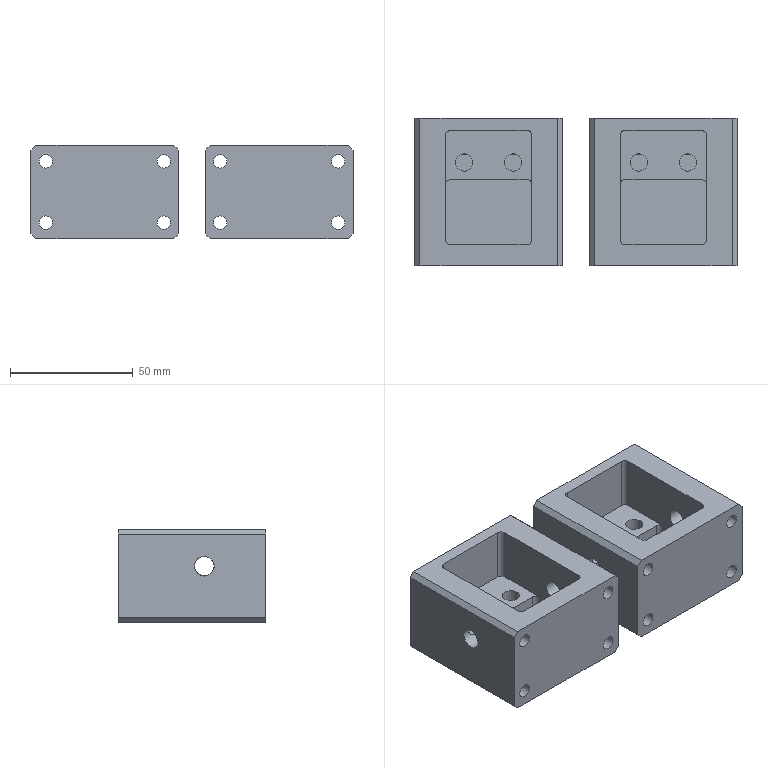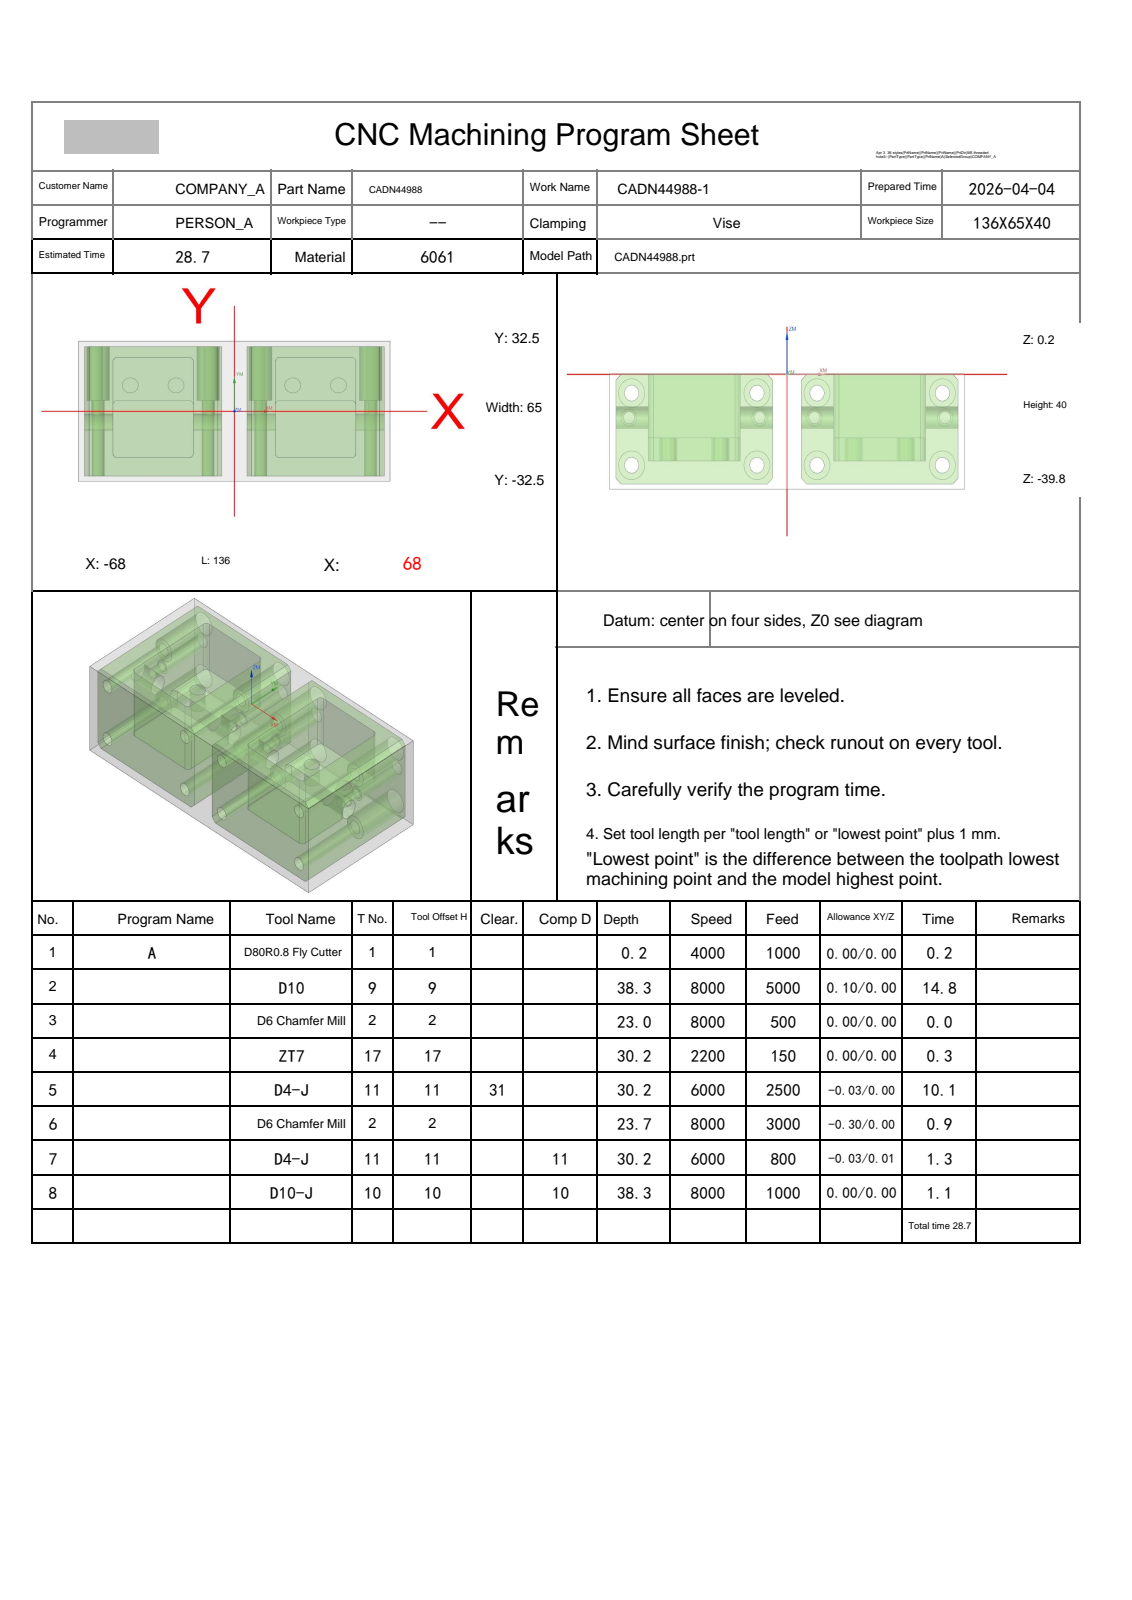NC program | NX | posted by the shop | part box 131 x 60 x 38 mm
Lines 4540 to 5571 of 30516:
N5 T11 M06
(D4-J  D=4. R=0. H=11 ce=0.00 di=0.01)
G00 G90 G54 X47.547 Y-18.9 M03 S6000
G43 H11 Z20.
M08
Z.303
G01 X47.548 Y-18.907 Z.217 F2000.
X47.551 Y-18.926 Z.139
X47.556 Y-18.955 Z.069
X47.564 Y-18.994 Z.007
X47.575 Y-19.039 Z-.049
X47.589 Y-19.09 Z-.098
X47.606 Y-19.144 Z-.141
X47.627 Y-19.2 Z-.177
X47.651 Y-19.256 Z-.208
X47.68 Y-19.31 Z-.234
X47.712 Y-19.361 Z-.255
X47.749 Y-19.406 Z-.271
X47.791 Y-19.445 Z-.283
X47.838 Y-19.474 Z-.291
X47.89 Y-19.493 Z-.296
X47.947 Y-19.5 Z-.297
X51.1 F2500.
Y-16.347
X51.084 Y-16.304 Z-.298
X51.038 Y-16.282 Z-.301
X50.966 Y-16.28 Z-.305
X50.871 Y-16.297 Z-.31
X50.756 Y-16.33 Z-.317
X50.626 Y-16.379 Z-.325
X50.482 Y-16.441 Z-.334
X50.33 Y-16.516 Z-.344
X50.171 Y-16.6 Z-.355
X50.01 Y-16.693 Z-.366
X49.85 Y-16.794 Z-.378
X49.512 Y-17.035 Z-.404
X49.197 Y-17.303 Z-.432
X48.905 Y-17.595 Z-.46
X48.638 Y-17.911 Z-.487
X48.397 Y-18.249 Z-.514
X48.296 Y-18.409 Z-.526
X48.202 Y-18.57 Z-.537
X48.117 Y-18.729 Z-.547
X48.043 Y-18.882 Z-.557
X47.98 Y-19.025 Z-.566
X47.931 Y-19.156 Z-.574
X47.898 Y-19.271 Z-.581
X47.881 Y-19.366 Z-.587
X47.882 Y-19.438 Z-.591
X47.904 Y-19.484 Z-.594
X47.947 Y-19.5
X51.1
Y-16.347
X51.084 Y-16.304 Z-.595
X51.038 Y-16.282 Z-.598
X50.966 Y-16.28 Z-.602
X50.871 Y-16.296 Z-.608
X50.756 Y-16.33 Z-.615
X50.626 Y-16.378 Z-.623
X50.482 Y-16.44 Z-.632
X50.329 Y-16.514 Z-.642
X50.171 Y-16.598 Z-.652
X50.01 Y-16.691 Z-.663
X49.85 Y-16.791 Z-.675
X49.512 Y-17.033 Z-.702
X49.197 Y-17.3 Z-.729
X48.905 Y-17.593 Z-.757
X48.638 Y-17.909 Z-.785
X48.397 Y-18.247 Z-.811
X48.296 Y-18.408 Z-.823
X48.202 Y-18.569 Z-.834
X48.117 Y-18.728 Z-.845
X48.043 Y-18.881 Z-.855
X47.98 Y-19.025 Z-.864
X47.931 Y-19.156 Z-.872
X47.898 Y-19.27 Z-.878
X47.881 Y-19.366 Z-.884
X47.882 Y-19.438 Z-.888
X47.904 Y-19.484 Z-.891
X47.947 Y-19.5 Z-.892
X51.1
Y-16.347
X51.084 Y-16.304 Z-.893
X51.038 Y-16.282 Z-.895
X50.966 Y-16.28 Z-.899
X50.871 Y-16.296 Z-.905
X50.756 Y-16.329 Z-.912
X50.625 Y-16.377 Z-.92
X50.482 Y-16.438 Z-.929
X50.329 Y-16.512 Z-.939
X50.171 Y-16.596 Z-.949
X50.01 Y-16.689 Z-.961
X49.85 Y-16.789 Z-.972
X49.512 Y-17.03 Z-.999
X49.197 Y-17.297 Z-1.026
X48.905 Y-17.59 Z-1.054
X48.638 Y-17.907 Z-1.082
X48.396 Y-18.246 Z-1.108
X48.296 Y-18.406 Z-1.12
X48.202 Y-18.568 Z-1.131
X48.117 Y-18.727 Z-1.142
X48.043 Y-18.88 Z-1.152
X47.98 Y-19.024 Z-1.161
X47.931 Y-19.155 Z-1.169
X47.898 Y-19.27 Z-1.176
X47.881 Y-19.366 Z-1.181
X47.882 Y-19.438 Z-1.185
X47.904 Y-19.484 Z-1.188
X47.947 Y-19.5 Z-1.189
X51.1
Y-16.347
X51.084 Y-16.304 Z-1.19
X51.038 Y-16.282 Z-1.192
X50.966 Y-16.279 Z-1.197
X50.871 Y-16.295 Z-1.202
X50.756 Y-16.328 Z-1.209
X50.625 Y-16.375 Z-1.217
X50.482 Y-16.436 Z-1.226
X50.329 Y-16.51 Z-1.236
X50.171 Y-16.593 Z-1.247
X50.01 Y-16.686 Z-1.258
X49.85 Y-16.786 Z-1.269
X49.512 Y-17.027 Z-1.296
X49.197 Y-17.295 Z-1.324
X48.905 Y-17.588 Z-1.351
X48.638 Y-17.905 Z-1.379
X48.396 Y-18.244 Z-1.406
X48.296 Y-18.405 Z-1.417
X48.202 Y-18.567 Z-1.428
X48.117 Y-18.726 Z-1.439
X48.043 Y-18.88 Z-1.449
X47.98 Y-19.024 Z-1.458
X47.931 Y-19.155 Z-1.466
X47.898 Y-19.27 Z-1.473
X47.881 Y-19.365 Z-1.478
X47.882 Y-19.438 Z-1.483
X47.904 Y-19.484 Z-1.485
X47.947 Y-19.5 Z-1.486
X51.1
Y-16.347
X51.084 Y-16.304
X51.038 Y-16.281 Z-1.487
X50.966 Y-16.279 Z-1.489
X50.871 Y-16.294 Z-1.492
X50.756 Y-16.327 Z-1.495
X50.625 Y-16.374 Z-1.499
X50.482 Y-16.435 Z-1.504
X50.329 Y-16.508 Z-1.511
X50.171 Y-16.591 Z-1.518
X50.01 Y-16.684 Z-1.526
X49.85 Y-16.783 Z-1.535
X49.512 Y-17.024 Z-1.56
X49.197 Y-17.292 Z-1.589
X48.905 Y-17.585 Z-1.62
X48.638 Y-17.903 Z-1.653
X48.396 Y-18.243 Z-1.685
X48.296 Y-18.404 Z-1.699
X48.202 Y-18.566 Z-1.713
X48.117 Y-18.725 Z-1.726
X48.043 Y-18.879 Z-1.738
X47.98 Y-19.023 Z-1.749
X47.931 Y-19.155 Z-1.759
X47.898 Y-19.27 Z-1.767
X47.881 Y-19.365 Z-1.774
X47.882 Y-19.438 Z-1.779
X47.904 Y-19.484 Z-1.782
X47.947 Y-19.5 Z-1.783
X51.1
Y-16.347
X51.084 Y-16.304 Z-1.784
X51.038 Y-16.281 Z-1.785
X50.966 Y-16.278 Z-1.786
X50.871 Y-16.294 Z-1.789
X50.756 Y-16.326 Z-1.792
X50.625 Y-16.373 Z-1.797
X50.482 Y-16.433 Z-1.802
X50.329 Y-16.506 Z-1.808
X50.171 Y-16.589 Z-1.815
X50.01 Y-16.681 Z-1.823
X49.85 Y-16.781 Z-1.833
X49.512 Y-17.021 Z-1.857
X49.197 Y-17.289 Z-1.886
X48.905 Y-17.583 Z-1.917
X48.638 Y-17.901 Z-1.95
X48.397 Y-18.241 Z-1.982
X48.296 Y-18.402 Z-1.997
X48.202 Y-18.565 Z-2.01
X48.117 Y-18.724 Z-2.023
X48.043 Y-18.878 Z-2.035
X47.98 Y-19.023 Z-2.046
X47.931 Y-19.154 Z-2.056
X47.898 Y-19.269 Z-2.064
X47.881 Y-19.365 Z-2.071
X47.882 Y-19.438 Z-2.076
X47.904 Y-19.484 Z-2.08
X47.947 Y-19.5 Z-2.081
X51.1
Y-16.347
X51.084 Y-16.303
X51.038 Y-16.281 Z-2.082
X50.966 Y-16.278 Z-2.084
X50.871 Y-16.293 Z-2.086
X50.756 Y-16.325 Z-2.09
X50.626 Y-16.371 Z-2.094
X50.482 Y-16.432 Z-2.099
X50.329 Y-16.504 Z-2.105
X50.171 Y-16.587 Z-2.112
X50.01 Y-16.679 Z-2.121
X49.85 Y-16.778 Z-2.13
X49.512 Y-17.018 Z-2.155
X49.197 Y-17.286 Z-2.183
X48.905 Y-17.58 Z-2.215
X48.638 Y-17.899 Z-2.247
X48.397 Y-18.24 Z-2.28
X48.25 Y-18.48 Z-2.301
X48.117 Y-18.723 Z-2.321
X48.043 Y-18.877 Z-2.333
X47.98 Y-19.022 Z-2.344
X47.931 Y-19.154 Z-2.353
X47.898 Y-19.269 Z-2.362
X47.881 Y-19.365 Z-2.369
X47.882 Y-19.438 Z-2.374
X47.904 Y-19.484 Z-2.377
X47.947 Y-19.5 Z-2.378
X51.1
Y-16.347
X51.084 Y-16.303
X51.038 Y-16.281 Z-2.379
X50.966 Y-16.278 Z-2.381
X50.871 Y-16.292 Z-2.383
X50.756 Y-16.324 Z-2.387
X50.626 Y-16.37 Z-2.391
X50.482 Y-16.43 Z-2.396
X50.329 Y-16.502 Z-2.403
X50.171 Y-16.584 Z-2.41
X50.01 Y-16.676 Z-2.418
X49.85 Y-16.775 Z-2.427
X49.512 Y-17.015 Z-2.452
X49.197 Y-17.283 Z-2.481
X48.905 Y-17.578 Z-2.512
X48.638 Y-17.896 Z-2.545
X48.397 Y-18.238 Z-2.577
X48.25 Y-18.479 Z-2.598
X48.117 Y-18.723 Z-2.618
X48.043 Y-18.877 Z-2.63
X47.98 Y-19.021 Z-2.641
X47.931 Y-19.153 Z-2.651
X47.898 Y-19.269 Z-2.659
X47.881 Y-19.365 Z-2.666
X47.882 Y-19.438 Z-2.671
X47.904 Y-19.484 Z-2.674
X47.947 Y-19.5 Z-2.675
X51.1
Y-16.347
X51.084 Y-16.303
X51.038 Y-16.281 Z-2.676
X50.966 Y-16.277 Z-2.678
X50.871 Y-16.292 Z-2.681
X50.756 Y-16.323 Z-2.684
X50.626 Y-16.369 Z-2.688
X50.482 Y-16.428 Z-2.694
X50.33 Y-16.5 Z-2.7
X50.171 Y-16.582 Z-2.707
X50.01 Y-16.673 Z-2.715
X49.85 Y-16.772 Z-2.725
X49.512 Y-17.012 Z-2.749
X49.197 Y-17.281 Z-2.778
X48.905 Y-17.575 Z-2.81
X48.638 Y-17.894 Z-2.842
X48.397 Y-18.236 Z-2.874
X48.25 Y-18.478 Z-2.895
X48.117 Y-18.722 Z-2.915
X48.043 Y-18.876 Z-2.927
X47.98 Y-19.021 Z-2.938
X47.931 Y-19.153 Z-2.948
X47.898 Y-19.269 Z-2.956
X47.881 Y-19.365 Z-2.963
X47.882 Y-19.438 Z-2.968
X47.904 Y-19.484 Z-2.971
X47.947 Y-19.5 Z-2.972
X51.1
Y-16.347
X51.084 Y-16.303 Z-2.973
X51.038 Y-16.28 Z-2.974
X50.966 Y-16.277 Z-2.975
X50.871 Y-16.291 Z-2.978
X50.756 Y-16.322 Z-2.981
X50.626 Y-16.367 Z-2.986
X50.482 Y-16.427 Z-2.991
X50.33 Y-16.498 Z-2.997
X50.171 Y-16.58 Z-3.004
X50.01 Y-16.671 Z-3.013
X49.85 Y-16.77 Z-3.022
X49.513 Y-17.009 Z-3.047
X49.197 Y-17.278 Z-3.075
X48.906 Y-17.573 Z-3.107
X48.638 Y-17.892 Z-3.139
X48.397 Y-18.235 Z-3.172
X48.25 Y-18.477 Z-3.192
X48.117 Y-18.721 Z-3.212
X48.043 Y-18.875 Z-3.224
X47.98 Y-19.02 Z-3.235
X47.931 Y-19.153 Z-3.245
X47.898 Y-19.268 Z-3.253
X47.881 Y-19.365 Z-3.26
X47.882 Y-19.438 Z-3.265
X47.904 Y-19.484 Z-3.268
X47.947 Y-19.5 Z-3.27
X51.1
Y-16.347
X51.084 Y-16.303
X51.038 Y-16.28 Z-3.271
X50.966 Y-16.276 Z-3.273
X50.871 Y-16.29 Z-3.275
X50.756 Y-16.321 Z-3.279
X50.626 Y-16.366 Z-3.283
X50.482 Y-16.425 Z-3.288
X50.33 Y-16.496 Z-3.295
X50.171 Y-16.577 Z-3.302
X50.01 Y-16.668 Z-3.31
X49.85 Y-16.767 Z-3.32
X49.513 Y-17.006 Z-3.344
X49.197 Y-17.275 Z-3.373
X48.906 Y-17.57 Z-3.404
X48.638 Y-17.89 Z-3.437
X48.397 Y-18.233 Z-3.469
X48.25 Y-18.475 Z-3.49
X48.117 Y-18.72 Z-3.51
X48.043 Y-18.875 Z-3.522
X47.98 Y-19.02 Z-3.533
X47.931 Y-19.152 Z-3.542
X47.898 Y-19.268 Z-3.551
X47.881 Y-19.364 Z-3.557
X47.882 Y-19.437 Z-3.563
X47.904 Y-19.484 Z-3.566
X47.947 Y-19.5 Z-3.567
X51.1
Y-16.347
X51.084 Y-16.303
X51.038 Y-16.28 Z-3.568
X50.966 Y-16.276 Z-3.57
X50.871 Y-16.29 Z-3.573
X50.756 Y-16.32 Z-3.576
X50.626 Y-16.365 Z-3.58
X50.482 Y-16.423 Z-3.586
X50.33 Y-16.494 Z-3.592
X50.171 Y-16.575 Z-3.599
X50.01 Y-16.666 Z-3.607
X49.85 Y-16.764 Z-3.617
X49.513 Y-17.003 Z-3.642
X49.198 Y-17.272 Z-3.67
X48.906 Y-17.568 Z-3.702
X48.638 Y-17.888 Z-3.734
X48.397 Y-18.232 Z-3.766
X48.25 Y-18.474 Z-3.787
X48.118 Y-18.719 Z-3.807
X48.043 Y-18.874 Z-3.819
X47.98 Y-19.019 Z-3.83
X47.931 Y-19.152 Z-3.84
X47.898 Y-19.268 Z-3.848
X47.881 Y-19.364 Z-3.855
X47.882 Y-19.437 Z-3.86
X47.904 Y-19.484 Z-3.863
X47.947 Y-19.5 Z-3.864
X51.1
Y-16.347
X51.084 Y-16.303
X51.038 Y-16.28 Z-3.865
X50.966 Y-16.276 Z-3.867
X50.871 Y-16.289 Z-3.87
X50.757 Y-16.319 Z-3.873
X50.626 Y-16.363 Z-3.878
X50.483 Y-16.421 Z-3.883
X50.33 Y-16.492 Z-3.889
X50.171 Y-16.573 Z-3.897
X50.011 Y-16.663 Z-3.905
X49.851 Y-16.761 Z-3.914
X49.513 Y-17. Z-3.939
X49.198 Y-17.269 Z-3.968
X48.906 Y-17.565 Z-3.999
X48.639 Y-17.886 Z-4.032
X48.397 Y-18.23 Z-4.064
X48.251 Y-18.473 Z-4.084
X48.118 Y-18.718 Z-4.104
X48.043 Y-18.873 Z-4.116
X47.98 Y-19.019 Z-4.127
X47.932 Y-19.151 Z-4.137
X47.898 Y-19.268 Z-4.145
X47.881 Y-19.364 Z-4.152
X47.882 Y-19.437 Z-4.157
X47.904 Y-19.484 Z-4.16
X47.947 Y-19.5 Z-4.161
X51.1
Y-16.347
X51.084 Y-16.303 Z-4.162
X51.038 Y-16.28 Z-4.163
X50.966 Y-16.275 Z-4.164
X50.871 Y-16.288 Z-4.167
X50.757 Y-16.318 Z-4.171
X50.626 Y-16.362 Z-4.175
X50.483 Y-16.42 Z-4.18
X50.33 Y-16.49 Z-4.187
X50.172 Y-16.57 Z-4.194
X50.011 Y-16.66 Z-4.202
X49.851 Y-16.758 Z-4.212
X49.513 Y-16.997 Z-4.236
X49.198 Y-17.266 Z-4.265
X48.906 Y-17.562 Z-4.296
X48.639 Y-17.884 Z-4.329
X48.397 Y-18.229 Z-4.361
X48.251 Y-18.472 Z-4.382
X48.118 Y-18.717 Z-4.402
X48.043 Y-18.872 Z-4.413
X47.981 Y-19.018 Z-4.424
X47.932 Y-19.151 Z-4.434
X47.898 Y-19.267 Z-4.442
X47.881 Y-19.364 Z-4.449
X47.882 Y-19.437 Z-4.454
X47.904 Y-19.484 Z-4.457
X47.947 Y-19.5 Z-4.458
X51.1
Y-16.347
X51.084 Y-16.303 Z-4.459
X51.038 Y-16.279 Z-4.46
X50.966 Y-16.275 Z-4.462
X50.871 Y-16.288 Z-4.464
X50.757 Y-16.317 Z-4.468
X50.626 Y-16.361 Z-4.472
X50.483 Y-16.418 Z-4.478
X50.33 Y-16.488 Z-4.484
X50.172 Y-16.568 Z-4.491
X50.011 Y-16.658 Z-4.5
X49.851 Y-16.756 Z-4.509
X49.513 Y-16.994 Z-4.534
X49.198 Y-17.263 Z-4.562
X48.906 Y-17.56 Z-4.594
X48.639 Y-17.882 Z-4.626
X48.397 Y-18.227 Z-4.658
X48.251 Y-18.47 Z-4.679
X48.118 Y-18.716 Z-4.699
X48.043 Y-18.872 Z-4.711
X47.981 Y-19.018 Z-4.722
X47.932 Y-19.151 Z-4.731
X47.898 Y-19.267 Z-4.74
X47.881 Y-19.364 Z-4.746
X47.882 Y-19.437 Z-4.751
X47.904 Y-19.484 Z-4.755
X47.947 Y-19.5 Z-4.756
X51.1
Y-16.347
X51.084 Y-16.303
X51.038 Y-16.279 Z-4.757
X50.966 Y-16.274 Z-4.759
X50.871 Y-16.287 Z-4.762
X50.757 Y-16.316 Z-4.765
X50.626 Y-16.359 Z-4.77
X50.483 Y-16.416 Z-4.775
X50.33 Y-16.486 Z-4.781
X50.172 Y-16.566 Z-4.789
X50.011 Y-16.655 Z-4.797
X49.851 Y-16.753 Z-4.807
X49.514 Y-16.991 Z-4.831
X49.198 Y-17.26 Z-4.86
X48.907 Y-17.557 Z-4.891
X48.639 Y-17.88 Z-4.924
X48.397 Y-18.225 Z-4.956
X48.251 Y-18.469 Z-4.976
X48.118 Y-18.715 Z-4.996
X48.043 Y-18.871 Z-5.008
X47.981 Y-19.017 Z-5.019
X47.932 Y-19.15 Z-5.029
X47.898 Y-19.267 Z-5.037
X47.881 Y-19.364 Z-5.044
X47.882 Y-19.437 Z-5.049
X47.904 Y-19.484 Z-5.052
X47.947 Y-19.5 Z-5.053
X51.1
Y-16.347
X51.084 Y-16.303
X51.038 Y-16.279 Z-5.054
X50.966 Y-16.274 Z-5.056
X50.871 Y-16.286 Z-5.059
X50.757 Y-16.315 Z-5.062
X50.626 Y-16.358 Z-5.067
X50.483 Y-16.415 Z-5.072
X50.331 Y-16.483 Z-5.079
X50.172 Y-16.563 Z-5.086
X50.011 Y-16.652 Z-5.094
X49.852 Y-16.75 Z-5.104
X49.514 Y-16.988 Z-5.129
X49.199 Y-17.257 Z-5.157
X48.907 Y-17.555 Z-5.189
X48.639 Y-17.877 Z-5.221
X48.397 Y-18.224 Z-5.253
X48.251 Y-18.468 Z-5.274
X48.118 Y-18.714 Z-5.293
X48.043 Y-18.87 Z-5.305
X47.981 Y-19.016 Z-5.316
X47.932 Y-19.15 Z-5.326
X47.898 Y-19.267 Z-5.334
X47.881 Y-19.364 Z-5.341
X47.882 Y-19.437 Z-5.346
X47.904 Y-19.484 Z-5.349
X47.947 Y-19.5 Z-5.35
X51.1
Y-16.347
X51.084 Y-16.303
X51.038 Y-16.279 Z-5.352
X50.966 Y-16.273 Z-5.353
X50.871 Y-16.285 Z-5.356
X50.757 Y-16.314 Z-5.36
X50.626 Y-16.356 Z-5.364
X50.483 Y-16.413 Z-5.37
X50.331 Y-16.481 Z-5.376
X50.172 Y-16.561 Z-5.383
X50.012 Y-16.65 Z-5.392
X49.852 Y-16.747 Z-5.401
X49.514 Y-16.985 Z-5.426
X49.199 Y-17.254 Z-5.455
X48.907 Y-17.552 Z-5.486
X48.64 Y-17.875 Z-5.518
X48.398 Y-18.222 Z-5.55
X48.251 Y-18.466 Z-5.571
X48.118 Y-18.713 Z-5.591
X48.043 Y-18.869 Z-5.603
X47.981 Y-19.016 Z-5.613
X47.932 Y-19.149 Z-5.623
X47.898 Y-19.266 Z-5.631
X47.881 Y-19.363 Z-5.638
X47.882 Y-19.437 Z-5.643
X47.904 Y-19.484 Z-5.646
X47.947 Y-19.5 Z-5.647
X51.1
Y-16.347
X51.084 Y-16.303 Z-5.648
X51.038 Y-16.279 Z-5.649
X50.966 Y-16.273 Z-5.651
X50.871 Y-16.285 Z-5.653
X50.757 Y-16.313 Z-5.657
X50.627 Y-16.355 Z-5.662
X50.483 Y-16.411 Z-5.667
X50.331 Y-16.479 Z-5.673
X50.173 Y-16.558 Z-5.681
X50.012 Y-16.647 Z-5.689
X49.852 Y-16.744 Z-5.699
X49.515 Y-16.982 Z-5.724
X49.199 Y-17.251 Z-5.752
X48.907 Y-17.549 Z-5.783
X48.64 Y-17.873 Z-5.816
X48.398 Y-18.22 Z-5.848
X48.251 Y-18.465 Z-5.868
X48.118 Y-18.712 Z-5.888
X48.043 Y-18.869 Z-5.9
X47.981 Y-19.015 Z-5.911
X47.932 Y-19.149 Z-5.92
X47.898 Y-19.266 Z-5.929
X47.881 Y-19.363 Z-5.935
X47.882 Y-19.437 Z-5.94
X47.904 Y-19.484 Z-5.944
X47.947 Y-19.5 Z-5.945
X51.1
Y-16.347
X51.084 Y-16.303
X51.038 Y-16.278 Z-5.946
X50.966 Y-16.273 Z-5.948
X50.872 Y-16.284 Z-5.951
X50.757 Y-16.312 Z-5.954
X50.627 Y-16.354 Z-5.959
X50.484 Y-16.409 Z-5.964
X50.331 Y-16.477 Z-5.971
X50.173 Y-16.556 Z-5.978
X50.012 Y-16.644 Z-5.987
X49.852 Y-16.741 Z-5.996
X49.515 Y-16.979 Z-6.021
X49.2 Y-17.248 Z-6.05
X48.908 Y-17.547 Z-6.081
X48.64 Y-17.871 Z-6.113
X48.398 Y-18.219 Z-6.145
X48.251 Y-18.464 Z-6.166
X48.118 Y-18.711 Z-6.185
X48.044 Y-18.868 Z-6.197
X47.981 Y-19.015 Z-6.208
X47.932 Y-19.149 Z-6.218
X47.898 Y-19.266 Z-6.226
X47.881 Y-19.363 Z-6.233
X47.882 Y-19.437 Z-6.238
X47.904 Y-19.484 Z-6.241
X47.947 Y-19.5 Z-6.242
X51.1
Y-16.347
X51.084 Y-16.303
X51.038 Y-16.278 Z-6.243
X50.966 Y-16.272 Z-6.245
X50.872 Y-16.283 Z-6.248
X50.757 Y-16.31 Z-6.252
X50.627 Y-16.352 Z-6.256
X50.484 Y-16.408 Z-6.262
X50.332 Y-16.475 Z-6.268
X50.173 Y-16.554 Z-6.276
X50.013 Y-16.642 Z-6.284
X49.853 Y-16.738 Z-6.294
X49.515 Y-16.976 Z-6.318
X49.2 Y-17.245 Z-6.347
X48.908 Y-17.544 Z-6.378
X48.64 Y-17.869 Z-6.41
X48.398 Y-18.217 Z-6.442
X48.252 Y-18.463 Z-6.463
X48.118 Y-18.71 Z-6.483
X48.044 Y-18.867 Z-6.494
X47.981 Y-19.014 Z-6.505
X47.932 Y-19.148 Z-6.515
X47.898 Y-19.266 Z-6.523
X47.881 Y-19.363 Z-6.53
X47.882 Y-19.437 Z-6.535
X47.904 Y-19.484 Z-6.538
X47.947 Y-19.5 Z-6.539
X51.1
Y-16.347
X51.084 Y-16.303
X51.038 Y-16.278 Z-6.541
X50.967 Y-16.272 Z-6.543
X50.872 Y-16.283 Z-6.545
X50.758 Y-16.309 Z-6.549
X50.627 Y-16.351 Z-6.554
X50.484 Y-16.406 Z-6.559
X50.332 Y-16.473 Z-6.566
X50.174 Y-16.551 Z-6.573
X50.013 Y-16.639 Z-6.582
X49.853 Y-16.735 Z-6.591
X49.516 Y-16.973 Z-6.616
X49.201 Y-17.242 Z-6.644
X48.908 Y-17.541 Z-6.676
X48.641 Y-17.867 Z-6.708
X48.398 Y-18.215 Z-6.74
X48.252 Y-18.461 Z-6.76
X48.118 Y-18.709 Z-6.78
X48.044 Y-18.866 Z-6.792
X47.981 Y-19.014 Z-6.803
X47.932 Y-19.148 Z-6.812
X47.898 Y-19.265 Z-6.82
X47.881 Y-19.363 Z-6.827
X47.882 Y-19.437 Z-6.832
X47.904 Y-19.484 Z-6.835
X47.947 Y-19.5 Z-6.836
X51.1
Y-16.347
X51.084 Y-16.303 Z-6.837
X51.038 Y-16.278 Z-6.838
X50.967 Y-16.271 Z-6.84
X50.872 Y-16.282 Z-6.843
X50.758 Y-16.308 Z-6.846
X50.627 Y-16.349 Z-6.851
X50.484 Y-16.404 Z-6.856
X50.332 Y-16.471 Z-6.863
X50.174 Y-16.549 Z-6.87
X50.013 Y-16.636 Z-6.879
X49.854 Y-16.732 Z-6.889
X49.516 Y-16.97 Z-6.913
X49.201 Y-17.239 Z-6.942
X48.909 Y-17.539 Z-6.973
X48.641 Y-17.864 Z-7.005
X48.399 Y-18.214 Z-7.037
X48.252 Y-18.46 Z-7.058
X48.119 Y-18.708 Z-7.077
X48.044 Y-18.866 Z-7.089
X47.981 Y-19.013 Z-7.1
X47.932 Y-19.147 Z-7.109
X47.898 Y-19.265 Z-7.118
X47.881 Y-19.363 Z-7.124
X47.882 Y-19.437 Z-7.129
X47.904 Y-19.484 Z-7.132
X47.947 Y-19.5 Z-7.134
X51.1
Y-16.347
X51.084 Y-16.303
X51.038 Y-16.278 Z-7.135
X50.967 Y-16.271 Z-7.137
X50.872 Y-16.281 Z-7.14
X50.758 Y-16.307 Z-7.144
X50.628 Y-16.348 Z-7.148
X50.485 Y-16.402 Z-7.154
X50.333 Y-16.469 Z-7.16
X50.174 Y-16.546 Z-7.168
X50.014 Y-16.633 Z-7.176
X49.854 Y-16.729 Z-7.186
X49.517 Y-16.966 Z-7.211
X49.202 Y-17.236 Z-7.239
X48.909 Y-17.536 Z-7.27
X48.641 Y-17.862 Z-7.303
X48.399 Y-18.212 Z-7.334
X48.252 Y-18.459 Z-7.355
X48.119 Y-18.707 Z-7.374
X48.044 Y-18.865 Z-7.386
X47.981 Y-19.012 Z-7.397
X47.932 Y-19.147 Z-7.407
X47.898 Y-19.265 Z-7.415
X47.881 Y-19.362 Z-7.422
X47.882 Y-19.437 Z-7.427
X47.904 Y-19.484 Z-7.43
X47.947 Y-19.5 Z-7.431
X51.1
Y-16.347
X51.084 Y-16.303
X51.039 Y-16.277 Z-7.432
X50.967 Y-16.27 Z-7.434
X50.872 Y-16.28 Z-7.437
X50.758 Y-16.306 Z-7.441
X50.628 Y-16.347 Z-7.446
X50.485 Y-16.401 Z-7.451
X50.333 Y-16.467 Z-7.458
X50.175 Y-16.544 Z-7.465
X50.014 Y-16.631 Z-7.474
X49.855 Y-16.726 Z-7.483
X49.517 Y-16.963 Z-7.508
X49.202 Y-17.233 Z-7.537
X48.91 Y-17.533 Z-7.568
X48.642 Y-17.86 Z-7.6
X48.399 Y-18.21 Z-7.632
X48.252 Y-18.457 Z-7.652
X48.119 Y-18.706 Z-7.672
X48.044 Y-18.864 Z-7.684
X47.981 Y-19.012 Z-7.694
X47.932 Y-19.146 Z-7.704
X47.898 Y-19.264 Z-7.712
X47.881 Y-19.362 Z-7.719
X47.882 Y-19.436 Z-7.724
X47.904 Y-19.484 Z-7.727
X47.947 Y-19.5 Z-7.728
X51.1
Y-16.347
X51.084 Y-16.302
X51.039 Y-16.277 Z-7.73
X50.967 Y-16.27 Z-7.732
X50.872 Y-16.28 Z-7.734
X50.758 Y-16.305 Z-7.738
X50.628 Y-16.345 Z-7.743
X50.485 Y-16.399 Z-7.748
X50.333 Y-16.464 Z-7.755
X50.175 Y-16.541 Z-7.763
X50.015 Y-16.628 Z-7.771
X49.855 Y-16.723 Z-7.781
X49.518 Y-16.96 Z-7.806
X49.203 Y-17.23 Z-7.834
X48.91 Y-17.531 Z-7.865
X48.642 Y-17.858 Z-7.897
X48.4 Y-18.209 Z-7.929
X48.253 Y-18.456 Z-7.95
X48.119 Y-18.705 Z-7.969
X48.044 Y-18.863 Z-7.981
X47.981 Y-19.011 Z-7.992
X47.932 Y-19.146 Z-8.001
X47.898 Y-19.264 Z-8.009
X47.881 Y-19.362 Z-8.016
X47.882 Y-19.436 Z-8.021
X47.904 Y-19.484 Z-8.024
X47.947 Y-19.5 Z-8.025
X51.1
Y-16.347
X51.084 Y-16.302 Z-8.026
X51.039 Y-16.277 Z-8.027
X50.967 Y-16.27 Z-8.029
X50.872 Y-16.279 Z-8.032
X50.758 Y-16.304 Z-8.036
X50.628 Y-16.344 Z-8.04
X50.486 Y-16.397 Z-8.046
X50.334 Y-16.462 Z-8.052
X50.176 Y-16.539 Z-8.06
X50.015 Y-16.625 Z-8.069
X49.856 Y-16.721 Z-8.078
X49.519 Y-16.957 Z-8.103
X49.203 Y-17.227 Z-8.132
X48.911 Y-17.528 Z-8.163
X48.643 Y-17.856 Z-8.195
X48.4 Y-18.207 Z-8.226
X48.253 Y-18.455 Z-8.247
X48.119 Y-18.704 Z-8.266
X48.044 Y-18.862 Z-8.278
X47.982 Y-19.011 Z-8.289
X47.932 Y-19.146 Z-8.298
X47.898 Y-19.264 Z-8.307
X47.881 Y-19.362 Z-8.313
X47.882 Y-19.436 Z-8.318
X47.904 Y-19.483 Z-8.321
X47.947 Y-19.5 Z-8.322
X51.1
Y-16.347
X51.084 Y-16.302 Z-8.323
X51.039 Y-16.277 Z-8.324
X50.967 Y-16.269 Z-8.326
X50.873 Y-16.278 Z-8.329
X50.759 Y-16.303 Z-8.333
X50.629 Y-16.342 Z-8.338
X50.486 Y-16.395 Z-8.343
X50.334 Y-16.46 Z-8.35
X50.176 Y-16.536 Z-8.357
X50.016 Y-16.622 Z-8.366
X49.856 Y-16.718 Z-8.376
X49.519 Y-16.954 Z-8.401
X49.204 Y-17.224 Z-8.429
X48.911 Y-17.525 Z-8.46
X48.643 Y-17.853 Z-8.492
X48.4 Y-18.205 Z-8.524
X48.253 Y-18.453 Z-8.544
X48.12 Y-18.704 Z-8.564
X48.045 Y-18.862 Z-8.575
X47.982 Y-19.01 Z-8.586
X47.932 Y-19.145 Z-8.596
X47.898 Y-19.264 Z-8.604
X47.881 Y-19.362 Z-8.611
X47.882 Y-19.436 Z-8.615
X47.904 Y-19.483 Z-8.619
X47.947 Y-19.5 Z-8.62
X51.1
Y-16.347
X51.084 Y-16.302
X51.039 Y-16.277 Z-8.621
X50.967 Y-16.269 Z-8.623
X50.873 Y-16.278 Z-8.626
X50.759 Y-16.302 Z-8.63
X50.629 Y-16.341 Z-8.635
X50.486 Y-16.393 Z-8.641
X50.335 Y-16.458 Z-8.647
X50.177 Y-16.534 Z-8.655
X50.017 Y-16.62 Z-8.664
X49.857 Y-16.715 Z-8.673
X49.52 Y-16.951 Z-8.698
X49.204 Y-17.221 Z-8.727
X48.912 Y-17.522 Z-8.758
X48.643 Y-17.851 Z-8.79
X48.401 Y-18.204 Z-8.821
X48.253 Y-18.452 Z-8.842
X48.12 Y-18.703 Z-8.861
X48.045 Y-18.861 Z-8.873
X47.982 Y-19.009 Z-8.883
X47.932 Y-19.145 Z-8.893
X47.898 Y-19.263 Z-8.901
X47.881 Y-19.362 Z-8.908
X47.882 Y-19.436 Z-8.913
X47.904 Y-19.483 Z-8.916
X47.947 Y-19.5 Z-8.917
X51.1
Y-16.347
X51.084 Y-16.302
X51.039 Y-16.276 Z-8.919
X50.967 Y-16.268 Z-8.921
X50.873 Y-16.277 Z-8.924
X50.759 Y-16.301 Z-8.927
X50.629 Y-16.34 Z-8.932
X50.487 Y-16.392 Z-8.938
X50.335 Y-16.456 Z-8.945
X50.177 Y-16.531 Z-8.952
X50.017 Y-16.617 Z-8.961
X49.858 Y-16.712 Z-8.971
X49.521 Y-16.947 Z-8.996
X49.205 Y-17.218 Z-9.024
X48.912 Y-17.52 Z-9.055
X48.644 Y-17.849 Z-9.087
X48.401 Y-18.202 Z-9.119
X48.254 Y-18.451 Z-9.139
X48.12 Y-18.702 Z-9.158
X48.045 Y-18.86 Z-9.17
X47.982 Y-19.009 Z-9.181
X47.933 Y-19.144 Z-9.19
X47.898 Y-19.263 Z-9.198
X47.881 Y-19.361 Z-9.205
X47.882 Y-19.436 Z-9.21
X47.904 Y-19.483 Z-9.213
X47.947 Y-19.5 Z-9.214
X51.1
Y-16.347
X51.084 Y-16.302 Z-9.215
X51.039 Y-16.276 Z-9.216
X50.967 Y-16.268 Z-9.218
X50.873 Y-16.276 Z-9.221
X50.759 Y-16.3 Z-9.225
X50.63 Y-16.338 Z-9.23
X50.487 Y-16.39 Z-9.235
X50.336 Y-16.454 Z-9.242
X50.178 Y-16.529 Z-9.25
X50.018 Y-16.614 Z-9.258
X49.858 Y-16.709 Z-9.268
X49.521 Y-16.944 Z-9.293
X49.206 Y-17.215 Z-9.322
X48.913 Y-17.517 Z-9.353
X48.645 Y-17.847 Z-9.384
X48.401 Y-18.2 Z-9.416
X48.254 Y-18.449 Z-9.436
X48.12 Y-18.701 Z-9.456
X48.045 Y-18.859 Z-9.467
X47.982 Y-19.008 Z-9.478
X47.933 Y-19.144 Z-9.487
X47.898 Y-19.263 Z-9.496
X47.881 Y-19.361 Z-9.502
X47.882 Y-19.436 Z-9.507
X47.904 Y-19.483 Z-9.51
X47.947 Y-19.5 Z-9.511
X51.1
Y-16.347
X51.084 Y-16.302 Z-9.512
X51.039 Y-16.276 Z-9.513
X50.967 Y-16.267 Z-9.515
X50.873 Y-16.275 Z-9.518
X50.76 Y-16.299 Z-9.522
X50.63 Y-16.337 Z-9.527
X50.488 Y-16.388 Z-9.533
X50.336 Y-16.452 Z-9.539
X50.179 Y-16.526 Z-9.547
X50.019 Y-16.611 Z-9.556
X49.859 Y-16.706 Z-9.566
X49.522 Y-16.941 Z-9.591
X49.207 Y-17.212 Z-9.619
X48.914 Y-17.514 Z-9.65
X48.645 Y-17.844 Z-9.682
X48.402 Y-18.199 Z-9.713
X48.254 Y-18.448 Z-9.734
X48.12 Y-18.7 Z-9.753
X48.045 Y-18.859 Z-9.765
X47.982 Y-19.008 Z-9.775
X47.933 Y-19.144 Z-9.785
X47.899 Y-19.263 Z-9.793
X47.881 Y-19.361 Z-9.8
X47.882 Y-19.436 Z-9.804
X47.904 Y-19.483 Z-9.808
X47.947 Y-19.5 Z-9.809
X51.1
Y-16.347
X51.084 Y-16.302
X51.039 Y-16.276 Z-9.81
X50.968 Y-16.267 Z-9.812
X50.873 Y-16.275 Z-9.815
X50.76 Y-16.298 Z-9.819
X50.63 Y-16.335 Z-9.824
X50.488 Y-16.386 Z-9.83
X50.337 Y-16.449 Z-9.837
X50.179 Y-16.524 Z-9.845
X50.019 Y-16.609 Z-9.853
X49.86 Y-16.703 Z-9.863
X49.523 Y-16.938 Z-9.888
X49.207 Y-17.209 Z-9.917
X48.915 Y-17.511 Z-9.947
X48.646 Y-17.842 Z-9.979
X48.402 Y-18.197 Z-10.011
X48.255 Y-18.447 Z-10.031
X48.121 Y-18.699 Z-10.05
X48.046 Y-18.858 Z-10.062
X47.982 Y-19.007 Z-10.073
X47.933 Y-19.143 Z-10.082
X47.899 Y-19.262 Z-10.09
X47.881 Y-19.361 Z-10.097
X47.883 Y-19.436 Z-10.102
X47.904 Y-19.483 Z-10.105
X47.947 Y-19.5 Z-10.106
X51.1
Y-16.347
X51.084 Y-16.302
X51.039 Y-16.276 Z-10.108
X50.968 Y-16.266 Z-10.11
X50.874 Y-16.274 Z-10.113
X50.76 Y-16.297 Z-10.117
X50.631 Y-16.334 Z-10.122
X50.489 Y-16.384 Z-10.127
X50.337 Y-16.447 Z-10.134
X50.18 Y-16.521 Z-10.142
X50.02 Y-16.606 Z-10.151
X49.861 Y-16.7 Z-10.161
X49.524 Y-16.935 Z-10.186
X49.208 Y-17.206 Z-10.214
X48.915 Y-17.509 Z-10.245
X48.646 Y-17.84 Z-10.277
X48.403 Y-18.195 Z-10.308
X48.255 Y-18.445 Z-10.328
X48.121 Y-18.698 Z-10.348
X48.046 Y-18.857 Z-10.359
X47.983 Y-19.007 Z-10.37
X47.933 Y-19.143 Z-10.379
X47.899 Y-19.262 Z-10.387
X47.881 Y-19.361 Z-10.394
X47.883 Y-19.436 Z-10.399
X47.904 Y-19.483 Z-10.402
X47.947 Y-19.5 Z-10.403
X51.1
Y-16.347
X51.084 Y-16.302
X51.039 Y-16.275 Z-10.405
X50.968 Y-16.266 Z-10.407
X50.874 Y-16.273 Z-10.41
X50.761 Y-16.296 Z-10.414
X50.631 Y-16.332 Z-10.419
X50.489 Y-16.383 Z-10.425
X50.338 Y-16.445 Z-10.432
X50.181 Y-16.519 Z-10.44
X50.021 Y-16.603 Z-10.448
X49.862 Y-16.697 Z-10.458
X49.525 Y-16.931 Z-10.483
X49.209 Y-17.203 Z-10.512
X48.916 Y-17.506 Z-10.542
X48.647 Y-17.838 Z-10.574
X48.403 Y-18.194 Z-10.605
X48.255 Y-18.444 Z-10.626
X48.121 Y-18.697 Z-10.645
X48.046 Y-18.856 Z-10.656
X47.983 Y-19.006 Z-10.667
X47.933 Y-19.142 Z-10.677
X47.899 Y-19.262 Z-10.685
X47.881 Y-19.361 Z-10.691
X47.883 Y-19.436 Z-10.696
X47.904 Y-19.483 Z-10.699
X47.947 Y-19.5 Z-10.7
X51.1
Y-16.347
X51.084 Y-16.302 Z-10.701
X51.039 Y-16.275 Z-10.702
X50.968 Y-16.266 Z-10.704
X50.874 Y-16.272 Z-10.707
X50.761 Y-16.294 Z-10.711
X50.632 Y-16.331 Z-10.716
X50.49 Y-16.381 Z-10.722
X50.339 Y-16.443 Z-10.729
X50.181 Y-16.516 Z-10.737
X50.022 Y-16.6 Z-10.746
X49.863 Y-16.694 Z-10.756
X49.526 Y-16.928 Z-10.781
X49.21 Y-17.199 Z-10.809
X48.917 Y-17.503 Z-10.84
X48.648 Y-17.835 Z-10.872
X48.404 Y-18.192 Z-10.903
X48.256 Y-18.443 Z-10.923
X48.122 Y-18.696 Z-10.942
X48.046 Y-18.855 Z-10.954
X47.983 Y-19.005 Z-10.964
X47.933 Y-19.142 Z-10.974
X47.899 Y-19.261 Z-10.982